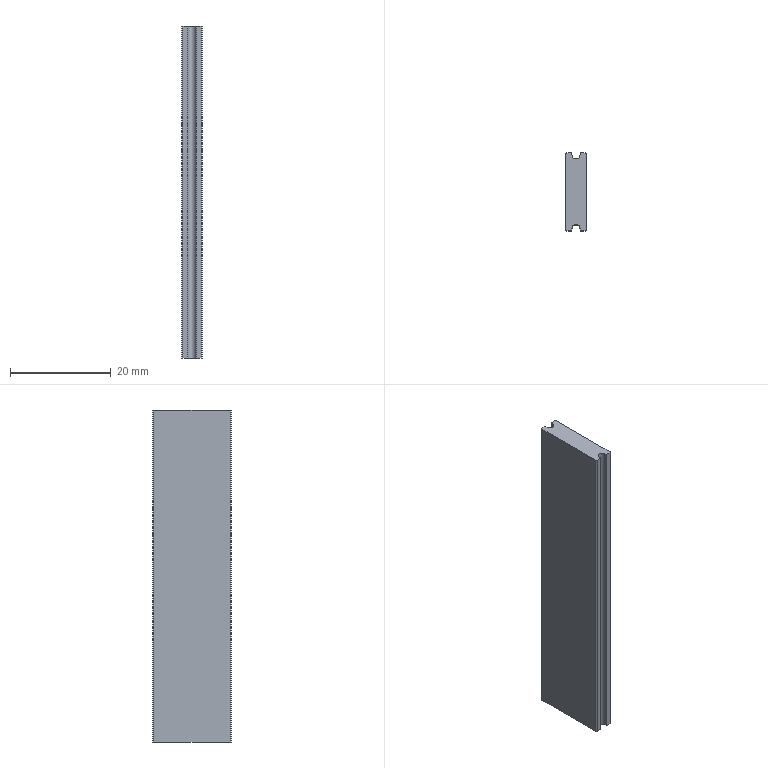Part | STEP file | LUOI DOT | 1 solid | 22 faces | box 4 x 15.5 x 65.8 mm | volume 3850 mm3 | plane 12 | cylinder 10 | commonest cylinder face diameters 0.2 x4 0.4 x4 1.6 x2